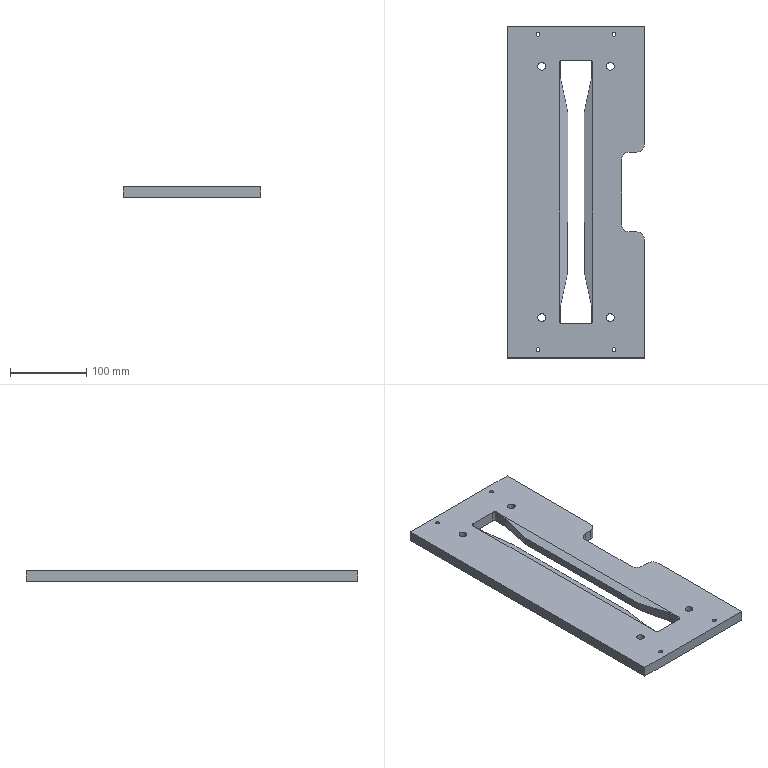Part | SolidWorks | features HoleWzd 2, ICE 2, Extrusion 1, Fillet 1 | 1 solid | 60 faces | box 180 x 436 x 14 mm | volume 907497 mm3 | cylinder 28 | plane 28 | cone 4 | commonest cylinder face diameters 5 x8 6 x8 10.2 x8 20 x4